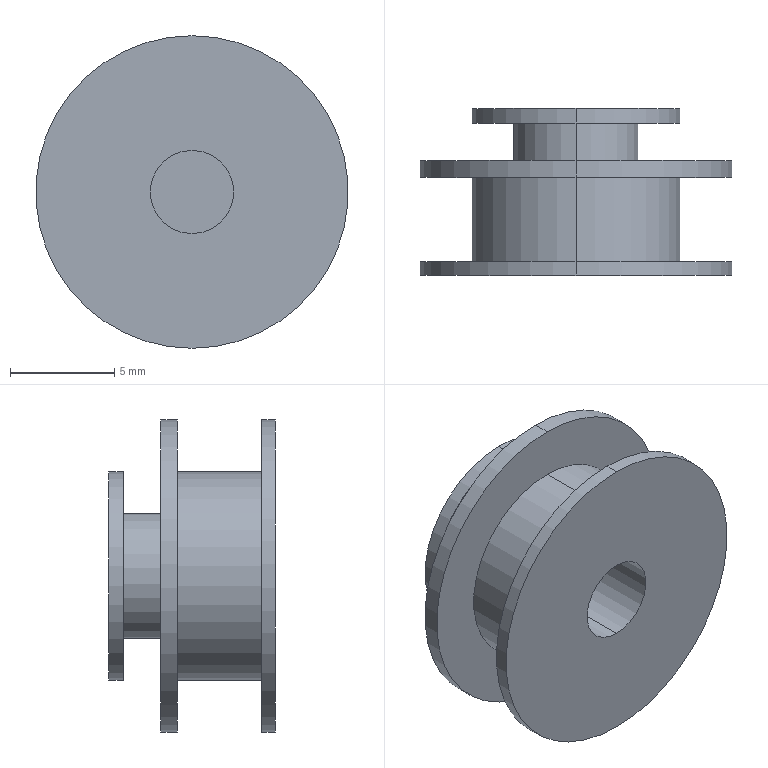Part | SolidWorks | features ICE 4, RevCut 2, Extrusion 1 | 1 solid | 22 faces | box 15 x 8 x 15 mm | volume 589.716 mm3 | cylinder 14 | plane 8 | commonest cylinder face diameters 4 x4 10 x4 15 x4 6 x2
STEP:
#1=CARTESIAN_POINT('',(0.,0.,-2.));
#2=VERTEX_POINT('',#1);
#3=CARTESIAN_POINT('',(0.,0.,2.));
#4=VERTEX_POINT('',#3);
#5=CARTESIAN_POINT('',(0.,0.,0.));
#6=DIRECTION('',(0.,1.,0.));
#7=DIRECTION('',(0.,0.,1.));
#8=AXIS2_PLACEMENT_3D('',#5,#6,#7);
#9=CIRCLE('',#8,2.);
#10=EDGE_CURVE('',#2,#4,#9,.T.);
#11=ORIENTED_EDGE('',*,*,#10,.F.);
#12=CARTESIAN_POINT('',(0.,4.7,-2.));
#13=VERTEX_POINT('',#12);
#14=CARTESIAN_POINT('',(0.,0.,-2.));
#15=DIRECTION('',(0.,1.,0.));
#16=VECTOR('',#15,1000.);
#17=LINE('',#14,#16);
#18=EDGE_CURVE('',#2,#13,#17,.T.);
#19=ORIENTED_EDGE('',*,*,#18,.T.);
#20=CARTESIAN_POINT('',(0.,4.7,2.));
#21=VERTEX_POINT('',#20);
#22=CARTESIAN_POINT('',(0.,4.7,0.));
#23=DIRECTION('',(0.,-1.,0.));
#24=DIRECTION('',(0.,0.,1.));
#25=AXIS2_PLACEMENT_3D('',#22,#23,#24);
#26=CIRCLE('',#25,2.);
#27=EDGE_CURVE('',#21,#13,#26,.T.);
#28=ORIENTED_EDGE('',*,*,#27,.F.);
#29=CARTESIAN_POINT('',(0.,0.,2.));
#30=DIRECTION('',(0.,1.,0.));
#31=VECTOR('',#30,1000.);
#32=LINE('',#29,#31);
#33=EDGE_CURVE('',#4,#21,#32,.T.);
#34=ORIENTED_EDGE('',*,*,#33,.F.);
#35=EDGE_LOOP('',(#11,#19,#28,#34));
#36=FACE_OUTER_BOUND('',#35,.T.);
#37=CARTESIAN_POINT('',(0.,0.,0.));
#38=DIRECTION('',(0.,1.,0.));
#39=DIRECTION('',(0.,0.,1.));
#40=AXIS2_PLACEMENT_3D('',#37,#38,#39);
#41=CYLINDRICAL_SURFACE('',#40,2.);
#42=ADVANCED_FACE('',(#36),#41,.F.);
#43=CARTESIAN_POINT('',(0.,0.65,-7.5));
#44=VERTEX_POINT('',#43);
#45=CARTESIAN_POINT('',(0.,0.65,7.5));
#46=VERTEX_POINT('',#45);
#47=CARTESIAN_POINT('',(0.,0.65,0.));
#48=DIRECTION('',(0.,-1.,0.));
#49=DIRECTION('',(0.,0.,-1.));
#50=AXIS2_PLACEMENT_3D('',#47,#48,#49);
#51=CIRCLE('',#50,7.5);
#52=EDGE_CURVE('',#44,#46,#51,.T.);
#53=ORIENTED_EDGE('',*,*,#52,.T.);
#54=CARTESIAN_POINT('',(0.,0.,7.5));
#55=VERTEX_POINT('',#54);
#56=CARTESIAN_POINT('',(0.,4.,7.5));
#57=DIRECTION('',(0.,-1.,0.));
#58=VECTOR('',#57,1000.);
#59=LINE('',#56,#58);
#60=EDGE_CURVE('',#46,#55,#59,.T.);
#61=ORIENTED_EDGE('',*,*,#60,.T.);
#62=CARTESIAN_POINT('',(0.,0.,-7.5));
#63=VERTEX_POINT('',#62);
#64=CARTESIAN_POINT('',(0.,0.,0.));
#65=DIRECTION('',(0.,1.,0.));
#66=DIRECTION('',(0.,0.,1.));
#67=AXIS2_PLACEMENT_3D('',#64,#65,#66);
#68=CIRCLE('',#67,7.5);
#69=EDGE_CURVE('',#55,#63,#68,.T.);
#70=ORIENTED_EDGE('',*,*,#69,.T.);
#71=CARTESIAN_POINT('',(0.,4.,-7.5));
#72=DIRECTION('',(0.,-1.,0.));
#73=VECTOR('',#72,1000.);
#74=LINE('',#71,#73);
#75=EDGE_CURVE('',#44,#63,#74,.T.);
#76=ORIENTED_EDGE('',*,*,#75,.F.);
#77=EDGE_LOOP('',(#53,#61,#70,#76));
#78=FACE_OUTER_BOUND('',#77,.T.);
#79=CARTESIAN_POINT('',(0.,4.,0.));
#80=DIRECTION('',(0.,-1.,0.));
#81=DIRECTION('',(0.,0.,-1.));
#82=AXIS2_PLACEMENT_3D('',#79,#80,#81);
#83=CYLINDRICAL_SURFACE('',#82,7.5);
#84=ADVANCED_FACE('',(#78),#83,.T.);
#85=CARTESIAN_POINT('',(0.,4.7,5.));
#86=VERTEX_POINT('',#85);
#87=CARTESIAN_POINT('',(0.,4.7,-5.));
#88=VERTEX_POINT('',#87);
#89=CARTESIAN_POINT('',(0.,4.7,0.));
#90=DIRECTION('',(0.,1.,0.));
#91=DIRECTION('',(0.,0.,1.));
#92=AXIS2_PLACEMENT_3D('',#89,#90,#91);
#93=CIRCLE('',#92,5.);
#94=EDGE_CURVE('',#86,#88,#93,.T.);
#95=ORIENTED_EDGE('',*,*,#94,.F.);
#96=CARTESIAN_POINT('',(0.,0.65,5.));
#97=VERTEX_POINT('',#96);
#98=CARTESIAN_POINT('',(0.,8.,5.));
#99=DIRECTION('',(0.,-1.,0.));
#100=VECTOR('',#99,1000.);
#101=LINE('',#98,#100);
#102=EDGE_CURVE('',#86,#97,#101,.T.);
#103=ORIENTED_EDGE('',*,*,#102,.T.);
#104=CARTESIAN_POINT('',(0.,0.65,-5.));
#105=VERTEX_POINT('',#104);
#106=CARTESIAN_POINT('',(0.,0.65,0.));
#107=DIRECTION('',(0.,1.,0.));
#108=DIRECTION('',(0.,0.,-1.));
#109=AXIS2_PLACEMENT_3D('',#106,#107,#108);
#110=CIRCLE('',#109,5.);
#111=EDGE_CURVE('',#97,#105,#110,.T.);
#112=ORIENTED_EDGE('',*,*,#111,.T.);
#113=CARTESIAN_POINT('',(0.,8.,-5.));
#114=DIRECTION('',(0.,-1.,0.));
#115=VECTOR('',#114,1000.);
#116=LINE('',#113,#115);
#117=EDGE_CURVE('',#88,#105,#116,.T.);
#118=ORIENTED_EDGE('',*,*,#117,.F.);
#119=EDGE_LOOP('',(#95,#103,#112,#118));
#120=FACE_OUTER_BOUND('',#119,.T.);
#121=CARTESIAN_POINT('',(0.,8.,0.));
#122=DIRECTION('',(0.,-1.,0.));
#123=DIRECTION('',(0.,0.,-1.));
#124=AXIS2_PLACEMENT_3D('',#121,#122,#123);
#125=CYLINDRICAL_SURFACE('',#124,5.);
#126=ADVANCED_FACE('',(#120),#125,.T.);
#127=CARTESIAN_POINT('',(0.,4.7,7.5));
#128=VERTEX_POINT('',#127);
#129=CARTESIAN_POINT('',(0.,4.7,-7.5));
#130=VERTEX_POINT('',#129);
#131=CARTESIAN_POINT('',(0.,4.7,0.));
#132=DIRECTION('',(0.,1.,0.));
#133=DIRECTION('',(0.,0.,1.));
#134=AXIS2_PLACEMENT_3D('',#131,#132,#133);
#135=CIRCLE('',#134,7.5);
#136=EDGE_CURVE('',#128,#130,#135,.T.);
#137=ORIENTED_EDGE('',*,*,#136,.T.);
#138=CARTESIAN_POINT('',(0.,5.5,-7.5));
#139=VERTEX_POINT('',#138);
#140=CARTESIAN_POINT('',(0.,4.7,-7.5));
#141=DIRECTION('',(0.,1.,0.));
#142=VECTOR('',#141,1000.);
#143=LINE('',#140,#142);
#144=EDGE_CURVE('',#130,#139,#143,.T.);
#145=ORIENTED_EDGE('',*,*,#144,.T.);
#146=CARTESIAN_POINT('',(0.,5.5,7.5));
#147=VERTEX_POINT('',#146);
#148=CARTESIAN_POINT('',(0.,5.5,0.));
#149=DIRECTION('',(0.,1.,0.));
#150=DIRECTION('',(0.,0.,1.));
#151=AXIS2_PLACEMENT_3D('',#148,#149,#150);
#152=CIRCLE('',#151,7.5);
#153=EDGE_CURVE('',#147,#139,#152,.T.);
#154=ORIENTED_EDGE('',*,*,#153,.F.);
#155=CARTESIAN_POINT('',(0.,4.7,7.5));
#156=DIRECTION('',(0.,1.,0.));
#157=VECTOR('',#156,1000.);
#158=LINE('',#155,#157);
#159=EDGE_CURVE('',#128,#147,#158,.T.);
#160=ORIENTED_EDGE('',*,*,#159,.F.);
#161=EDGE_LOOP('',(#137,#145,#154,#160));
#162=FACE_OUTER_BOUND('',#161,.T.);
#163=CARTESIAN_POINT('',(0.,4.7,0.));
#164=DIRECTION('',(0.,1.,0.));
#165=DIRECTION('',(0.,0.,1.));
#166=AXIS2_PLACEMENT_3D('',#163,#164,#165);
#167=CYLINDRICAL_SURFACE('',#166,7.5);
#168=ADVANCED_FACE('',(#162),#167,.T.);
#169=CARTESIAN_POINT('',(0.,5.5,2.));
#170=VERTEX_POINT('',#169);
#171=CARTESIAN_POINT('',(0.,5.5,-2.));
#172=VERTEX_POINT('',#171);
#173=CARTESIAN_POINT('',(0.,5.5,0.));
#174=DIRECTION('',(0.,-1.,0.));
#175=DIRECTION('',(0.,0.,1.));
#176=AXIS2_PLACEMENT_3D('',#173,#174,#175);
#177=CIRCLE('',#176,2.);
#178=EDGE_CURVE('',#170,#172,#177,.T.);
#179=ORIENTED_EDGE('',*,*,#178,.T.);
#180=CARTESIAN_POINT('',(0.,8.,-2.));
#181=VERTEX_POINT('',#180);
#182=CARTESIAN_POINT('',(0.,0.,-2.));
#183=DIRECTION('',(0.,1.,0.));
#184=VECTOR('',#183,1000.);
#185=LINE('',#182,#184);
#186=EDGE_CURVE('',#172,#181,#185,.T.);
#187=ORIENTED_EDGE('',*,*,#186,.T.);
#188=CARTESIAN_POINT('',(0.,8.,2.));
#189=VERTEX_POINT('',#188);
#190=CARTESIAN_POINT('',(0.,8.,0.));
#191=DIRECTION('',(0.,1.,0.));
#192=DIRECTION('',(0.,0.,1.));
#193=AXIS2_PLACEMENT_3D('',#190,#191,#192);
#194=CIRCLE('',#193,2.);
#195=EDGE_CURVE('',#181,#189,#194,.T.);
#196=ORIENTED_EDGE('',*,*,#195,.T.);
#197=CARTESIAN_POINT('',(0.,0.,2.));
#198=DIRECTION('',(0.,1.,0.));
#199=VECTOR('',#198,1000.);
#200=LINE('',#197,#199);
#201=EDGE_CURVE('',#170,#189,#200,.T.);
#202=ORIENTED_EDGE('',*,*,#201,.F.);
#203=EDGE_LOOP('',(#179,#187,#196,#202));
#204=FACE_OUTER_BOUND('',#203,.T.);
#205=CARTESIAN_POINT('',(0.,0.,0.));
#206=DIRECTION('',(0.,1.,0.));
#207=DIRECTION('',(0.,0.,1.));
#208=AXIS2_PLACEMENT_3D('',#205,#206,#207);
#209=CYLINDRICAL_SURFACE('',#208,2.);
#210=ADVANCED_FACE('',(#204),#209,.F.);
#211=CARTESIAN_POINT('',(0.,8.,5.));
#212=VERTEX_POINT('',#211);
#213=CARTESIAN_POINT('',(0.,8.,-5.));
#214=VERTEX_POINT('',#213);
#215=CARTESIAN_POINT('',(0.,8.,0.));
#216=DIRECTION('',(0.,1.,0.));
#217=DIRECTION('',(0.,0.,1.));
#218=AXIS2_PLACEMENT_3D('',#215,#216,#217);
#219=CIRCLE('',#218,5.);
#220=EDGE_CURVE('',#212,#214,#219,.T.);
#221=ORIENTED_EDGE('',*,*,#220,.F.);
#222=CARTESIAN_POINT('',(0.,7.3,5.));
#223=VERTEX_POINT('',#222);
#224=CARTESIAN_POINT('',(0.,8.,5.));
#225=DIRECTION('',(0.,-1.,0.));
#226=VECTOR('',#225,1000.);
#227=LINE('',#224,#226);
#228=EDGE_CURVE('',#212,#223,#227,.T.);
#229=ORIENTED_EDGE('',*,*,#228,.T.);
#230=CARTESIAN_POINT('',(0.,7.3,-5.));
#231=VERTEX_POINT('',#230);
#232=CARTESIAN_POINT('',(0.,7.3,0.));
#233=DIRECTION('',(0.,-1.,0.));
#234=DIRECTION('',(0.,0.,-1.));
#235=AXIS2_PLACEMENT_3D('',#232,#233,#234);
#236=CIRCLE('',#235,5.);
#237=EDGE_CURVE('',#231,#223,#236,.T.);
#238=ORIENTED_EDGE('',*,*,#237,.F.);
#239=CARTESIAN_POINT('',(0.,8.,-5.));
#240=DIRECTION('',(0.,-1.,0.));
#241=VECTOR('',#240,1000.);
#242=LINE('',#239,#241);
#243=EDGE_CURVE('',#214,#231,#242,.T.);
#244=ORIENTED_EDGE('',*,*,#243,.F.);
#245=EDGE_LOOP('',(#221,#229,#238,#244));
#246=FACE_OUTER_BOUND('',#245,.T.);
#247=CARTESIAN_POINT('',(0.,8.,0.));
#248=DIRECTION('',(0.,-1.,0.));
#249=DIRECTION('',(0.,0.,-1.));
#250=AXIS2_PLACEMENT_3D('',#247,#248,#249);
#251=CYLINDRICAL_SURFACE('',#250,5.);
#252=ADVANCED_FACE('',(#246),#251,.T.);
#253=CARTESIAN_POINT('',(0.,7.3,-3.));
#254=VERTEX_POINT('',#253);
#255=CARTESIAN_POINT('',(0.,7.3,3.));
#256=VERTEX_POINT('',#255);
#257=CARTESIAN_POINT('',(0.,7.3,0.));
#258=DIRECTION('',(0.,-1.,0.));
#259=DIRECTION('',(0.,0.,-1.));
#260=AXIS2_PLACEMENT_3D('',#257,#258,#259);
#261=CIRCLE('',#260,3.);
#262=EDGE_CURVE('',#254,#256,#261,.T.);
#263=ORIENTED_EDGE('',*,*,#262,.T.);
#264=CARTESIAN_POINT('',(0.,5.5,3.));
#265=VERTEX_POINT('',#264);
#266=CARTESIAN_POINT('',(0.,4.,3.));
#267=DIRECTION('',(0.,-1.,0.));
#268=VECTOR('',#267,1000.);
#269=LINE('',#266,#268);
#270=EDGE_CURVE('',#256,#265,#269,.T.);
#271=ORIENTED_EDGE('',*,*,#270,.T.);
#272=CARTESIAN_POINT('',(0.,5.5,-3.));
#273=VERTEX_POINT('',#272);
#274=CARTESIAN_POINT('',(0.,5.5,0.));
#275=DIRECTION('',(0.,-1.,0.));
#276=DIRECTION('',(0.,0.,-1.));
#277=AXIS2_PLACEMENT_3D('',#274,#275,#276);
#278=CIRCLE('',#277,3.);
#279=EDGE_CURVE('',#273,#265,#278,.T.);
#280=ORIENTED_EDGE('',*,*,#279,.F.);
#281=CARTESIAN_POINT('',(0.,4.,-3.));
#282=DIRECTION('',(0.,-1.,0.));
#283=VECTOR('',#282,1000.);
#284=LINE('',#281,#283);
#285=EDGE_CURVE('',#254,#273,#284,.T.);
#286=ORIENTED_EDGE('',*,*,#285,.F.);
#287=EDGE_LOOP('',(#263,#271,#280,#286));
#288=FACE_OUTER_BOUND('',#287,.T.);
#289=CARTESIAN_POINT('',(0.,4.,0.));
#290=DIRECTION('',(0.,-1.,0.));
#291=DIRECTION('',(0.,0.,-1.));
#292=AXIS2_PLACEMENT_3D('',#289,#290,#291);
#293=CYLINDRICAL_SURFACE('',#292,3.);
#294=ADVANCED_FACE('',(#288),#293,.T.);
#295=ORIENTED_EDGE('',*,*,#262,.F.);
#296=CARTESIAN_POINT('',(0.,7.3,0.));
#297=DIRECTION('',(0.,-1.,0.));
#298=DIRECTION('',(0.,0.,-1.));
#299=AXIS2_PLACEMENT_3D('',#296,#297,#298);
#300=CIRCLE('',#299,3.);
#301=EDGE_CURVE('',#256,#254,#300,.T.);
#302=ORIENTED_EDGE('',*,*,#301,.F.);
#303=EDGE_LOOP('',(#295,#302));
#304=FACE_BOUND('',#303,.T.);
#305=ORIENTED_EDGE('',*,*,#237,.T.);
#306=CARTESIAN_POINT('',(0.,7.3,0.));
#307=DIRECTION('',(0.,-1.,0.));
#308=DIRECTION('',(0.,0.,-1.));
#309=AXIS2_PLACEMENT_3D('',#306,#307,#308);
#310=CIRCLE('',#309,5.);
#311=EDGE_CURVE('',#223,#231,#310,.T.);
#312=ORIENTED_EDGE('',*,*,#311,.T.);
#313=EDGE_LOOP('',(#305,#312));
#314=FACE_OUTER_BOUND('',#313,.T.);
#315=CARTESIAN_POINT('',(5.,7.3,0.));
#316=DIRECTION('',(0.,1.,0.));
#317=DIRECTION('',(0.,0.,1.));
#318=AXIS2_PLACEMENT_3D('',#315,#316,#317);
#319=PLANE('',#318);
#320=ADVANCED_FACE('',(#304,#314),#319,.F.);
#321=ORIENTED_EDGE('',*,*,#270,.F.);
#322=ORIENTED_EDGE('',*,*,#301,.T.);
#323=ORIENTED_EDGE('',*,*,#285,.T.);
#324=CARTESIAN_POINT('',(0.,5.5,0.));
#325=DIRECTION('',(0.,-1.,0.));
#326=DIRECTION('',(0.,0.,-1.));
#327=AXIS2_PLACEMENT_3D('',#324,#325,#326);
#328=CIRCLE('',#327,3.);
#329=EDGE_CURVE('',#265,#273,#328,.T.);
#330=ORIENTED_EDGE('',*,*,#329,.F.);
#331=EDGE_LOOP('',(#321,#322,#323,#330));
#332=FACE_OUTER_BOUND('',#331,.T.);
#333=CARTESIAN_POINT('',(0.,4.,0.));
#334=DIRECTION('',(0.,-1.,0.));
#335=DIRECTION('',(0.,0.,-1.));
#336=AXIS2_PLACEMENT_3D('',#333,#334,#335);
#337=CYLINDRICAL_SURFACE('',#336,3.);
#338=ADVANCED_FACE('',(#332),#337,.T.);
#339=ORIENTED_EDGE('',*,*,#279,.T.);
#340=ORIENTED_EDGE('',*,*,#329,.T.);
#341=EDGE_LOOP('',(#339,#340));
#342=FACE_BOUND('',#341,.T.);
#343=ORIENTED_EDGE('',*,*,#153,.T.);
#344=CARTESIAN_POINT('',(0.,5.5,0.));
#345=DIRECTION('',(0.,1.,0.));
#346=DIRECTION('',(0.,0.,1.));
#347=AXIS2_PLACEMENT_3D('',#344,#345,#346);
#348=CIRCLE('',#347,7.5);
#349=EDGE_CURVE('',#139,#147,#348,.T.);
#350=ORIENTED_EDGE('',*,*,#349,.T.);
#351=EDGE_LOOP('',(#343,#350));
#352=FACE_OUTER_BOUND('',#351,.T.);
#353=CARTESIAN_POINT('',(5.,5.5,0.));
#354=DIRECTION('',(0.,-1.,0.));
#355=DIRECTION('',(0.,0.,-1.));
#356=AXIS2_PLACEMENT_3D('',#353,#354,#355);
#357=PLANE('',#356);
#358=ADVANCED_FACE('',(#342,#352),#357,.F.);
#359=CARTESIAN_POINT('',(0.,8.,0.));
#360=DIRECTION('',(0.,1.,0.));
#361=DIRECTION('',(0.,0.,1.));
#362=AXIS2_PLACEMENT_3D('',#359,#360,#361);
#363=CIRCLE('',#362,2.);
#364=EDGE_CURVE('',#189,#181,#363,.T.);
#365=ORIENTED_EDGE('',*,*,#364,.F.);
#366=ORIENTED_EDGE('',*,*,#195,.F.);
#367=EDGE_LOOP('',(#365,#366));
#368=FACE_BOUND('',#367,.T.);
#369=CARTESIAN_POINT('',(0.,8.,0.));
#370=DIRECTION('',(0.,1.,0.));
#371=DIRECTION('',(0.,0.,1.));
#372=AXIS2_PLACEMENT_3D('',#369,#370,#371);
#373=CIRCLE('',#372,5.);
#374=EDGE_CURVE('',#214,#212,#373,.T.);
#375=ORIENTED_EDGE('',*,*,#374,.T.);
#376=ORIENTED_EDGE('',*,*,#220,.T.);
#377=EDGE_LOOP('',(#375,#376));
#378=FACE_OUTER_BOUND('',#377,.T.);
#379=CARTESIAN_POINT('',(0.,8.,0.));
#380=DIRECTION('',(0.,1.,0.));
#381=DIRECTION('',(0.,0.,1.));
#382=AXIS2_PLACEMENT_3D('',#379,#380,#381);
#383=PLANE('',#382);
#384=ADVANCED_FACE('',(#368,#378),#383,.T.);
#385=ORIENTED_EDGE('',*,*,#228,.F.);
#386=ORIENTED_EDGE('',*,*,#374,.F.);
#387=ORIENTED_EDGE('',*,*,#243,.T.);
#388=ORIENTED_EDGE('',*,*,#311,.F.);
#389=EDGE_LOOP('',(#385,#386,#387,#388));
#390=FACE_OUTER_BOUND('',#389,.T.);
#391=CARTESIAN_POINT('',(0.,8.,0.));
#392=DIRECTION('',(0.,-1.,0.));
#393=DIRECTION('',(0.,0.,-1.));
#394=AXIS2_PLACEMENT_3D('',#391,#392,#393);
#395=CYLINDRICAL_SURFACE('',#394,5.);
#396=ADVANCED_FACE('',(#390),#395,.T.);
#397=ORIENTED_EDGE('',*,*,#186,.F.);
#398=CARTESIAN_POINT('',(0.,5.5,0.));
#399=DIRECTION('',(0.,-1.,0.));
#400=DIRECTION('',(0.,0.,1.));
#401=AXIS2_PLACEMENT_3D('',#398,#399,#400);
#402=CIRCLE('',#401,2.);
#403=EDGE_CURVE('',#172,#170,#402,.T.);
#404=ORIENTED_EDGE('',*,*,#403,.T.);
#405=ORIENTED_EDGE('',*,*,#201,.T.);
#406=ORIENTED_EDGE('',*,*,#364,.T.);
#407=EDGE_LOOP('',(#397,#404,#405,#406));
#408=FACE_OUTER_BOUND('',#407,.T.);
#409=CARTESIAN_POINT('',(0.,0.,0.));
#410=DIRECTION('',(0.,1.,0.));
#411=DIRECTION('',(0.,0.,1.));
#412=AXIS2_PLACEMENT_3D('',#409,#410,#411);
#413=CYLINDRICAL_SURFACE('',#412,2.);
#414=ADVANCED_FACE('',(#408),#413,.F.);
#415=ORIENTED_EDGE('',*,*,#178,.F.);
#416=ORIENTED_EDGE('',*,*,#403,.F.);
#417=EDGE_LOOP('',(#415,#416));
#418=FACE_OUTER_BOUND('',#417,.T.);
#419=CARTESIAN_POINT('',(0.,5.5,0.));
#420=DIRECTION('',(0.,1.,0.));
#421=DIRECTION('',(0.,0.,1.));
#422=AXIS2_PLACEMENT_3D('',#419,#420,#421);
#423=PLANE('',#422);
#424=ADVANCED_FACE('',(#418),#423,.T.);
#425=ORIENTED_EDGE('',*,*,#136,.F.);
#426=CARTESIAN_POINT('',(0.,4.7,0.));
#427=DIRECTION('',(0.,1.,0.));
#428=DIRECTION('',(0.,0.,1.));
#429=AXIS2_PLACEMENT_3D('',#426,#427,#428);
#430=CIRCLE('',#429,7.5);
#431=EDGE_CURVE('',#130,#128,#430,.T.);
#432=ORIENTED_EDGE('',*,*,#431,.F.);
#433=EDGE_LOOP('',(#425,#432));
#434=FACE_OUTER_BOUND('',#433,.T.);
#435=CARTESIAN_POINT('',(0.,4.7,0.));
#436=DIRECTION('',(0.,1.,0.));
#437=DIRECTION('',(0.,0.,1.));
#438=AXIS2_PLACEMENT_3D('',#435,#436,#437);
#439=CIRCLE('',#438,5.);
#440=EDGE_CURVE('',#88,#86,#439,.T.);
#441=ORIENTED_EDGE('',*,*,#440,.T.);
#442=ORIENTED_EDGE('',*,*,#94,.T.);
#443=EDGE_LOOP('',(#441,#442));
#444=FACE_BOUND('',#443,.T.);
#445=CARTESIAN_POINT('',(0.,4.7,0.));
#446=DIRECTION('',(0.,1.,0.));
#447=DIRECTION('',(0.,0.,1.));
#448=AXIS2_PLACEMENT_3D('',#445,#446,#447);
#449=PLANE('',#448);
#450=ADVANCED_FACE('',(#434,#444),#449,.F.);
#451=ORIENTED_EDGE('',*,*,#144,.F.);
#452=ORIENTED_EDGE('',*,*,#431,.T.);
#453=ORIENTED_EDGE('',*,*,#159,.T.);
#454=ORIENTED_EDGE('',*,*,#349,.F.);
#455=EDGE_LOOP('',(#451,#452,#453,#454));
#456=FACE_OUTER_BOUND('',#455,.T.);
#457=CARTESIAN_POINT('',(0.,4.7,0.));
#458=DIRECTION('',(0.,1.,0.));
#459=DIRECTION('',(0.,0.,1.));
#460=AXIS2_PLACEMENT_3D('',#457,#458,#459);
#461=CYLINDRICAL_SURFACE('',#460,7.5);
#462=ADVANCED_FACE('',(#456),#461,.T.);
#463=CARTESIAN_POINT('',(0.,0.65,0.));
#464=DIRECTION('',(0.,1.,0.));
#465=DIRECTION('',(0.,0.,-1.));
#466=AXIS2_PLACEMENT_3D('',#463,#464,#465);
#467=CIRCLE('',#466,5.);
#468=EDGE_CURVE('',#105,#97,#467,.T.);
#469=ORIENTED_EDGE('',*,*,#468,.F.);
#470=ORIENTED_EDGE('',*,*,#111,.F.);
#471=EDGE_LOOP('',(#469,#470));
#472=FACE_BOUND('',#471,.T.);
#473=ORIENTED_EDGE('',*,*,#52,.F.);
#474=CARTESIAN_POINT('',(0.,0.65,0.));
#475=DIRECTION('',(0.,-1.,0.));
#476=DIRECTION('',(0.,0.,-1.));
#477=AXIS2_PLACEMENT_3D('',#474,#475,#476);
#478=CIRCLE('',#477,7.5);
#479=EDGE_CURVE('',#46,#44,#478,.T.);
#480=ORIENTED_EDGE('',*,*,#479,.F.);
#481=EDGE_LOOP('',(#473,#480));
#482=FACE_OUTER_BOUND('',#481,.T.);
#483=CARTESIAN_POINT('',(7.5,0.65,0.));
#484=DIRECTION('',(0.,-1.,0.));
#485=DIRECTION('',(0.,0.,-1.));
#486=AXIS2_PLACEMENT_3D('',#483,#484,#485);
#487=PLANE('',#486);
#488=ADVANCED_FACE('',(#472,#482),#487,.F.);
#489=ORIENTED_EDGE('',*,*,#102,.F.);
#490=ORIENTED_EDGE('',*,*,#440,.F.);
#491=ORIENTED_EDGE('',*,*,#117,.T.);
#492=ORIENTED_EDGE('',*,*,#468,.T.);
#493=EDGE_LOOP('',(#489,#490,#491,#492));
#494=FACE_OUTER_BOUND('',#493,.T.);
#495=CARTESIAN_POINT('',(0.,8.,0.));
#496=DIRECTION('',(0.,-1.,0.));
#497=DIRECTION('',(0.,0.,-1.));
#498=AXIS2_PLACEMENT_3D('',#495,#496,#497);
#499=CYLINDRICAL_SURFACE('',#498,5.);
#500=ADVANCED_FACE('',(#494),#499,.T.);
#501=ORIENTED_EDGE('',*,*,#60,.F.);
#502=ORIENTED_EDGE('',*,*,#479,.T.);
#503=ORIENTED_EDGE('',*,*,#75,.T.);
#504=CARTESIAN_POINT('',(0.,0.,0.));
#505=DIRECTION('',(0.,1.,0.));
#506=DIRECTION('',(0.,0.,1.));
#507=AXIS2_PLACEMENT_3D('',#504,#505,#506);
#508=CIRCLE('',#507,7.5);
#509=EDGE_CURVE('',#63,#55,#508,.T.);
#510=ORIENTED_EDGE('',*,*,#509,.T.);
#511=EDGE_LOOP('',(#501,#502,#503,#510));
#512=FACE_OUTER_BOUND('',#511,.T.);
#513=CARTESIAN_POINT('',(0.,4.,0.));
#514=DIRECTION('',(0.,-1.,0.));
#515=DIRECTION('',(0.,0.,-1.));
#516=AXIS2_PLACEMENT_3D('',#513,#514,#515);
#517=CYLINDRICAL_SURFACE('',#516,7.5);
#518=ADVANCED_FACE('',(#512),#517,.T.);
#519=CARTESIAN_POINT('',(0.,0.,0.));
#520=DIRECTION('',(0.,1.,0.));
#521=DIRECTION('',(0.,0.,1.));
#522=AXIS2_PLACEMENT_3D('',#519,#520,#521);
#523=CIRCLE('',#522,2.);
#524=EDGE_CURVE('',#4,#2,#523,.T.);
#525=ORIENTED_EDGE('',*,*,#524,.T.);
#526=ORIENTED_EDGE('',*,*,#10,.T.);
#527=EDGE_LOOP('',(#525,#526));
#528=FACE_BOUND('',#527,.T.);
#529=ORIENTED_EDGE('',*,*,#509,.F.);
#530=ORIENTED_EDGE('',*,*,#69,.F.);
#531=EDGE_LOOP('',(#529,#530));
#532=FACE_OUTER_BOUND('',#531,.T.);
#533=CARTESIAN_POINT('',(0.,0.,0.));
#534=DIRECTION('',(0.,1.,0.));
#535=DIRECTION('',(0.,0.,1.));
#536=AXIS2_PLACEMENT_3D('',#533,#534,#535);
#537=PLANE('',#536);
#538=ADVANCED_FACE('',(#528,#532),#537,.F.);
#539=ORIENTED_EDGE('',*,*,#18,.F.);
#540=ORIENTED_EDGE('',*,*,#524,.F.);
#541=ORIENTED_EDGE('',*,*,#33,.T.);
#542=CARTESIAN_POINT('',(0.,4.7,0.));
#543=DIRECTION('',(0.,-1.,0.));
#544=DIRECTION('',(0.,0.,1.));
#545=AXIS2_PLACEMENT_3D('',#542,#543,#544);
#546=CIRCLE('',#545,2.);
#547=EDGE_CURVE('',#13,#21,#546,.T.);
#548=ORIENTED_EDGE('',*,*,#547,.F.);
#549=EDGE_LOOP('',(#539,#540,#541,#548));
#550=FACE_OUTER_BOUND('',#549,.T.);
#551=CARTESIAN_POINT('',(0.,0.,0.));
#552=DIRECTION('',(0.,1.,0.));
#553=DIRECTION('',(0.,0.,1.));
#554=AXIS2_PLACEMENT_3D('',#551,#552,#553);
#555=CYLINDRICAL_SURFACE('',#554,2.);
#556=ADVANCED_FACE('',(#550),#555,.F.);
#557=ORIENTED_EDGE('',*,*,#27,.T.);
#558=ORIENTED_EDGE('',*,*,#547,.T.);
#559=EDGE_LOOP('',(#557,#558));
#560=FACE_OUTER_BOUND('',#559,.T.);
#561=CARTESIAN_POINT('',(0.,4.7,0.));
#562=DIRECTION('',(0.,1.,0.));
#563=DIRECTION('',(0.,0.,1.));
#564=AXIS2_PLACEMENT_3D('',#561,#562,#563);
#565=PLANE('',#564);
#566=ADVANCED_FACE('',(#560),#565,.F.);
#567=CLOSED_SHELL('',(#42,#84,#126,#168,#210,#252,#294,#320,#338,#358,#384,#396,#414,#424,#450,#462,#488,#500,#518,#538,#556,#566));
#568=MANIFOLD_SOLID_BREP('',#567);
#569=CARTESIAN_POINT('',(0.,0.,0.));
#570=DIRECTION('',(0.,0.,1.));
#571=DIRECTION('',(1.,0.,0.));
#572=AXIS2_PLACEMENT_3D('',#569,#570,#571);
#573=(LENGTH_UNIT()NAMED_UNIT(*)SI_UNIT(.MILLI.,.METRE.));
#574=UNCERTAINTY_MEASURE_WITH_UNIT(LENGTH_MEASURE(0.00001),#573,'','');
#575=(NAMED_UNIT(*)PLANE_ANGLE_UNIT()SI_UNIT($,.RADIAN.));
#576=(NAMED_UNIT(*)SI_UNIT($,.STERADIAN.)SOLID_ANGLE_UNIT());
#577=(GEOMETRIC_REPRESENTATION_CONTEXT(3)GLOBAL_UNCERTAINTY_ASSIGNED_CONTEXT((#574))GLOBAL_UNIT_ASSIGNED_CONTEXT((#573,#575,#576))REPRESENTATION_CONTEXT('',''));
#578=ADVANCED_BREP_SHAPE_REPRESENTATION('',(#568,#572),#577);